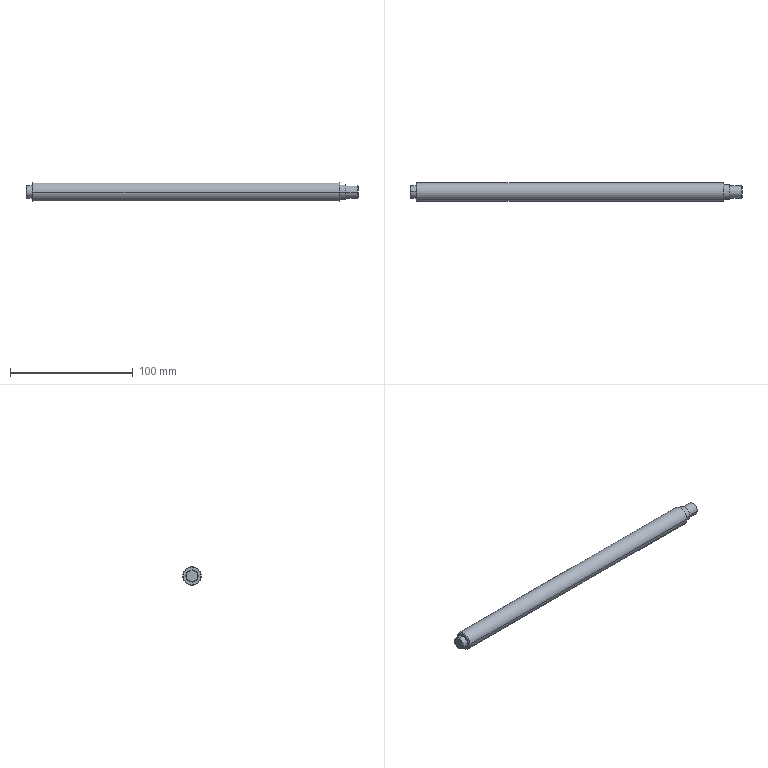Part | STEP file | Guide wheel mechanism revised.sldasm-Part-351 | 1 solid | 19 faces | box 270 x 15 x 15 mm | volume 45909 mm3 | cylinder 8 | cone 6 | plane 5 | commonest cylinder face diameters 10 x4 12 x2 15 x2
STEP:
#1=CARTESIAN_POINT('',(0.,0.,4.5));
#2=VERTEX_POINT('',#1);
#3=CARTESIAN_POINT('',(0.,0.,-4.5));
#4=VERTEX_POINT('',#3);
#5=CARTESIAN_POINT('',(0.,0.,0.));
#6=DIRECTION('',(-1.,0.,0.));
#7=DIRECTION('',(0.,1.,0.));
#8=AXIS2_PLACEMENT_3D('',#5,#6,#7);
#9=CIRCLE('',#8,4.5);
#10=EDGE_CURVE('',#2,#4,#9,.T.);
#11=ORIENTED_EDGE('',*,*,#10,.F.);
#12=CARTESIAN_POINT('',(0.5,0.,5.));
#13=VERTEX_POINT('',#12);
#14=CARTESIAN_POINT('',(0.,0.,4.5));
#15=DIRECTION('',(0.7071,0.,0.7071));
#16=VECTOR('',#15,1000.);
#17=LINE('',#14,#16);
#18=EDGE_CURVE('',#2,#13,#17,.T.);
#19=ORIENTED_EDGE('',*,*,#18,.T.);
#20=CARTESIAN_POINT('',(0.5,0.,-5.));
#21=VERTEX_POINT('',#20);
#22=CARTESIAN_POINT('',(0.5,0.,0.));
#23=DIRECTION('',(1.,0.,0.));
#24=DIRECTION('',(0.,0.,-1.));
#25=AXIS2_PLACEMENT_3D('',#22,#23,#24);
#26=CIRCLE('',#25,5.);
#27=EDGE_CURVE('',#21,#13,#26,.T.);
#28=ORIENTED_EDGE('',*,*,#27,.F.);
#29=CARTESIAN_POINT('',(0.,0.,-4.5));
#30=DIRECTION('',(0.7071,0.,-0.7071));
#31=VECTOR('',#30,1000.);
#32=LINE('',#29,#31);
#33=EDGE_CURVE('',#4,#21,#32,.T.);
#34=ORIENTED_EDGE('',*,*,#33,.F.);
#35=EDGE_LOOP('',(#11,#19,#28,#34));
#36=FACE_OUTER_BOUND('',#35,.T.);
#37=CARTESIAN_POINT('',(0.,0.,0.));
#38=DIRECTION('',(1.,0.,0.));
#39=DIRECTION('',(0.,0.,-1.));
#40=AXIS2_PLACEMENT_3D('',#37,#38,#39);
#41=CONICAL_SURFACE('',#40,4.5,0.7854);
#42=ADVANCED_FACE('',(#36),#41,.T.);
#43=CARTESIAN_POINT('',(5.,-7.,0.));
#44=VERTEX_POINT('',#43);
#45=CARTESIAN_POINT('',(5.,7.,0.));
#46=VERTEX_POINT('',#45);
#47=CARTESIAN_POINT('',(5.,0.,0.));
#48=DIRECTION('',(-1.,0.,0.));
#49=DIRECTION('',(0.,0.,1.));
#50=AXIS2_PLACEMENT_3D('',#47,#48,#49);
#51=CIRCLE('',#50,7.);
#52=EDGE_CURVE('',#44,#46,#51,.T.);
#53=ORIENTED_EDGE('',*,*,#52,.F.);
#54=CARTESIAN_POINT('',(5.5,-7.5,0.));
#55=VERTEX_POINT('',#54);
#56=CARTESIAN_POINT('',(5.,-7.,0.));
#57=DIRECTION('',(0.7071,-0.7071,0.));
#58=VECTOR('',#57,1000.);
#59=LINE('',#56,#58);
#60=EDGE_CURVE('',#44,#55,#59,.T.);
#61=ORIENTED_EDGE('',*,*,#60,.T.);
#62=CARTESIAN_POINT('',(5.5,7.5,0.));
#63=VERTEX_POINT('',#62);
#64=CARTESIAN_POINT('',(5.5,0.,0.));
#65=DIRECTION('',(1.,0.,0.));
#66=DIRECTION('',(0.,-1.,0.));
#67=AXIS2_PLACEMENT_3D('',#64,#65,#66);
#68=CIRCLE('',#67,7.5);
#69=EDGE_CURVE('',#63,#55,#68,.T.);
#70=ORIENTED_EDGE('',*,*,#69,.F.);
#71=CARTESIAN_POINT('',(5.,7.,0.));
#72=DIRECTION('',(0.7071,0.7071,0.));
#73=VECTOR('',#72,1000.);
#74=LINE('',#71,#73);
#75=EDGE_CURVE('',#46,#63,#74,.T.);
#76=ORIENTED_EDGE('',*,*,#75,.F.);
#77=EDGE_LOOP('',(#53,#61,#70,#76));
#78=FACE_OUTER_BOUND('',#77,.T.);
#79=CARTESIAN_POINT('',(5.,0.,0.));
#80=DIRECTION('',(1.,0.,0.));
#81=DIRECTION('',(0.,1.,0.));
#82=AXIS2_PLACEMENT_3D('',#79,#80,#81);
#83=CONICAL_SURFACE('',#82,7.,0.7854);
#84=ADVANCED_FACE('',(#78),#83,.T.);
#85=CARTESIAN_POINT('',(270.,4.5,0.));
#86=VERTEX_POINT('',#85);
#87=CARTESIAN_POINT('',(270.,-4.5,0.));
#88=VERTEX_POINT('',#87);
#89=CARTESIAN_POINT('',(270.,0.,0.));
#90=DIRECTION('',(1.,0.,0.));
#91=DIRECTION('',(0.,-1.,0.));
#92=AXIS2_PLACEMENT_3D('',#89,#90,#91);
#93=CIRCLE('',#92,4.5);
#94=EDGE_CURVE('',#86,#88,#93,.T.);
#95=ORIENTED_EDGE('',*,*,#94,.F.);
#96=CARTESIAN_POINT('',(269.5,5.,0.));
#97=VERTEX_POINT('',#96);
#98=CARTESIAN_POINT('',(269.5,5.,0.));
#99=DIRECTION('',(-0.7071,0.7071,0.));
#100=VECTOR('',#99,1000.);
#101=LINE('',#98,#100);
#102=EDGE_CURVE('',#86,#97,#101,.T.);
#103=ORIENTED_EDGE('',*,*,#102,.T.);
#104=CARTESIAN_POINT('',(269.5,-5.,0.));
#105=VERTEX_POINT('',#104);
#106=CARTESIAN_POINT('',(269.5,0.,0.));
#107=DIRECTION('',(-1.,0.,0.));
#108=DIRECTION('',(0.,-1.,0.));
#109=AXIS2_PLACEMENT_3D('',#106,#107,#108);
#110=CIRCLE('',#109,5.);
#111=EDGE_CURVE('',#105,#97,#110,.T.);
#112=ORIENTED_EDGE('',*,*,#111,.F.);
#113=CARTESIAN_POINT('',(269.5,-5.,0.));
#114=DIRECTION('',(-0.7071,-0.7071,0.));
#115=VECTOR('',#114,1000.);
#116=LINE('',#113,#115);
#117=EDGE_CURVE('',#88,#105,#116,.T.);
#118=ORIENTED_EDGE('',*,*,#117,.F.);
#119=EDGE_LOOP('',(#95,#103,#112,#118));
#120=FACE_OUTER_BOUND('',#119,.T.);
#121=CARTESIAN_POINT('',(269.5,0.,0.));
#122=DIRECTION('',(-1.,0.,0.));
#123=DIRECTION('',(0.,-1.,0.));
#124=AXIS2_PLACEMENT_3D('',#121,#122,#123);
#125=CONICAL_SURFACE('',#124,5.,0.7854);
#126=ADVANCED_FACE('',(#120),#125,.T.);
#127=CARTESIAN_POINT('',(5.,0.,5.));
#128=VERTEX_POINT('',#127);
#129=CARTESIAN_POINT('',(5.,0.,-5.));
#130=VERTEX_POINT('',#129);
#131=CARTESIAN_POINT('',(5.,0.,0.));
#132=DIRECTION('',(-1.,0.,0.));
#133=DIRECTION('',(0.,0.,1.));
#134=AXIS2_PLACEMENT_3D('',#131,#132,#133);
#135=CIRCLE('',#134,5.);
#136=EDGE_CURVE('',#128,#130,#135,.T.);
#137=ORIENTED_EDGE('',*,*,#136,.T.);
#138=CARTESIAN_POINT('',(12.,0.,-5.));
#139=DIRECTION('',(-1.,0.,0.));
#140=VECTOR('',#139,1000.);
#141=LINE('',#138,#140);
#142=EDGE_CURVE('',#130,#21,#141,.T.);
#143=ORIENTED_EDGE('',*,*,#142,.T.);
#144=ORIENTED_EDGE('',*,*,#27,.T.);
#145=CARTESIAN_POINT('',(12.,0.,5.));
#146=DIRECTION('',(-1.,0.,0.));
#147=VECTOR('',#146,1000.);
#148=LINE('',#145,#147);
#149=EDGE_CURVE('',#128,#13,#148,.T.);
#150=ORIENTED_EDGE('',*,*,#149,.F.);
#151=EDGE_LOOP('',(#137,#143,#144,#150));
#152=FACE_OUTER_BOUND('',#151,.T.);
#153=CARTESIAN_POINT('',(12.,0.,0.));
#154=DIRECTION('',(-1.,0.,0.));
#155=DIRECTION('',(0.,0.,1.));
#156=AXIS2_PLACEMENT_3D('',#153,#154,#155);
#157=CYLINDRICAL_SURFACE('',#156,5.);
#158=ADVANCED_FACE('',(#152),#157,.T.);
#159=ORIENTED_EDGE('',*,*,#111,.T.);
#160=CARTESIAN_POINT('',(260.,5.,0.));
#161=VERTEX_POINT('',#160);
#162=CARTESIAN_POINT('',(270.,5.,0.));
#163=DIRECTION('',(-1.,0.,0.));
#164=VECTOR('',#163,1000.);
#165=LINE('',#162,#164);
#166=EDGE_CURVE('',#97,#161,#165,.T.);
#167=ORIENTED_EDGE('',*,*,#166,.T.);
#168=CARTESIAN_POINT('',(260.,-5.,0.));
#169=VERTEX_POINT('',#168);
#170=CARTESIAN_POINT('',(260.,0.,0.));
#171=DIRECTION('',(-1.,0.,0.));
#172=DIRECTION('',(0.,-1.,0.));
#173=AXIS2_PLACEMENT_3D('',#170,#171,#172);
#174=CIRCLE('',#173,5.);
#175=EDGE_CURVE('',#169,#161,#174,.T.);
#176=ORIENTED_EDGE('',*,*,#175,.F.);
#177=CARTESIAN_POINT('',(270.,-5.,0.));
#178=DIRECTION('',(-1.,0.,0.));
#179=VECTOR('',#178,1000.);
#180=LINE('',#177,#179);
#181=EDGE_CURVE('',#105,#169,#180,.T.);
#182=ORIENTED_EDGE('',*,*,#181,.F.);
#183=EDGE_LOOP('',(#159,#167,#176,#182));
#184=FACE_OUTER_BOUND('',#183,.T.);
#185=CARTESIAN_POINT('',(270.,0.,0.));
#186=DIRECTION('',(-1.,0.,0.));
#187=DIRECTION('',(0.,-1.,0.));
#188=AXIS2_PLACEMENT_3D('',#185,#186,#187);
#189=CYLINDRICAL_SURFACE('',#188,5.);
#190=ADVANCED_FACE('',(#184),#189,.T.);
#191=CARTESIAN_POINT('',(260.,-6.,0.));
#192=VERTEX_POINT('',#191);
#193=CARTESIAN_POINT('',(260.,6.,0.));
#194=VERTEX_POINT('',#193);
#195=CARTESIAN_POINT('',(260.,0.,0.));
#196=DIRECTION('',(-1.,0.,0.));
#197=DIRECTION('',(0.,-1.,0.));
#198=AXIS2_PLACEMENT_3D('',#195,#196,#197);
#199=CIRCLE('',#198,6.);
#200=EDGE_CURVE('',#192,#194,#199,.T.);
#201=ORIENTED_EDGE('',*,*,#200,.T.);
#202=CARTESIAN_POINT('',(255.,6.,0.));
#203=VERTEX_POINT('',#202);
#204=CARTESIAN_POINT('',(270.,6.,0.));
#205=DIRECTION('',(-1.,0.,0.));
#206=VECTOR('',#205,1000.);
#207=LINE('',#204,#206);
#208=EDGE_CURVE('',#194,#203,#207,.T.);
#209=ORIENTED_EDGE('',*,*,#208,.T.);
#210=CARTESIAN_POINT('',(255.,-6.,0.));
#211=VERTEX_POINT('',#210);
#212=CARTESIAN_POINT('',(255.,0.,0.));
#213=DIRECTION('',(-1.,0.,0.));
#214=DIRECTION('',(0.,-1.,0.));
#215=AXIS2_PLACEMENT_3D('',#212,#213,#214);
#216=CIRCLE('',#215,6.);
#217=EDGE_CURVE('',#211,#203,#216,.T.);
#218=ORIENTED_EDGE('',*,*,#217,.F.);
#219=CARTESIAN_POINT('',(270.,-6.,0.));
#220=DIRECTION('',(-1.,0.,0.));
#221=VECTOR('',#220,1000.);
#222=LINE('',#219,#221);
#223=EDGE_CURVE('',#192,#211,#222,.T.);
#224=ORIENTED_EDGE('',*,*,#223,.F.);
#225=EDGE_LOOP('',(#201,#209,#218,#224));
#226=FACE_OUTER_BOUND('',#225,.T.);
#227=CARTESIAN_POINT('',(270.,0.,0.));
#228=DIRECTION('',(-1.,0.,0.));
#229=DIRECTION('',(0.,-1.,0.));
#230=AXIS2_PLACEMENT_3D('',#227,#228,#229);
#231=CYLINDRICAL_SURFACE('',#230,6.);
#232=ADVANCED_FACE('',(#226),#231,.T.);
#233=CARTESIAN_POINT('',(255.,-7.5,0.));
#234=VERTEX_POINT('',#233);
#235=CARTESIAN_POINT('',(255.,7.5,0.));
#236=VERTEX_POINT('',#235);
#237=CARTESIAN_POINT('',(255.,0.,0.));
#238=DIRECTION('',(-1.,0.,0.));
#239=DIRECTION('',(0.,-1.,0.));
#240=AXIS2_PLACEMENT_3D('',#237,#238,#239);
#241=CIRCLE('',#240,7.5);
#242=EDGE_CURVE('',#234,#236,#241,.T.);
#243=ORIENTED_EDGE('',*,*,#242,.T.);
#244=CARTESIAN_POINT('',(270.,7.5,0.));
#245=DIRECTION('',(-1.,0.,0.));
#246=VECTOR('',#245,1000.);
#247=LINE('',#244,#246);
#248=EDGE_CURVE('',#236,#63,#247,.T.);
#249=ORIENTED_EDGE('',*,*,#248,.T.);
#250=ORIENTED_EDGE('',*,*,#69,.T.);
#251=CARTESIAN_POINT('',(270.,-7.5,0.));
#252=DIRECTION('',(-1.,0.,0.));
#253=VECTOR('',#252,1000.);
#254=LINE('',#251,#253);
#255=EDGE_CURVE('',#234,#55,#254,.T.);
#256=ORIENTED_EDGE('',*,*,#255,.F.);
#257=EDGE_LOOP('',(#243,#249,#250,#256));
#258=FACE_OUTER_BOUND('',#257,.T.);
#259=CARTESIAN_POINT('',(270.,0.,0.));
#260=DIRECTION('',(-1.,0.,0.));
#261=DIRECTION('',(0.,-1.,0.));
#262=AXIS2_PLACEMENT_3D('',#259,#260,#261);
#263=CYLINDRICAL_SURFACE('',#262,7.5);
#264=ADVANCED_FACE('',(#258),#263,.T.);
#265=ORIENTED_EDGE('',*,*,#248,.F.);
#266=CARTESIAN_POINT('',(255.,0.,0.));
#267=DIRECTION('',(-1.,0.,0.));
#268=DIRECTION('',(0.,-1.,0.));
#269=AXIS2_PLACEMENT_3D('',#266,#267,#268);
#270=CIRCLE('',#269,7.5);
#271=EDGE_CURVE('',#236,#234,#270,.T.);
#272=ORIENTED_EDGE('',*,*,#271,.T.);
#273=ORIENTED_EDGE('',*,*,#255,.T.);
#274=CARTESIAN_POINT('',(5.5,0.,0.));
#275=DIRECTION('',(1.,0.,0.));
#276=DIRECTION('',(0.,-1.,0.));
#277=AXIS2_PLACEMENT_3D('',#274,#275,#276);
#278=CIRCLE('',#277,7.5);
#279=EDGE_CURVE('',#55,#63,#278,.T.);
#280=ORIENTED_EDGE('',*,*,#279,.T.);
#281=EDGE_LOOP('',(#265,#272,#273,#280));
#282=FACE_OUTER_BOUND('',#281,.T.);
#283=CARTESIAN_POINT('',(270.,0.,0.));
#284=DIRECTION('',(-1.,0.,0.));
#285=DIRECTION('',(0.,-1.,0.));
#286=AXIS2_PLACEMENT_3D('',#283,#284,#285);
#287=CYLINDRICAL_SURFACE('',#286,7.5);
#288=ADVANCED_FACE('',(#282),#287,.T.);
#289=ORIENTED_EDGE('',*,*,#242,.F.);
#290=ORIENTED_EDGE('',*,*,#271,.F.);
#291=EDGE_LOOP('',(#289,#290));
#292=FACE_OUTER_BOUND('',#291,.T.);
#293=ORIENTED_EDGE('',*,*,#217,.T.);
#294=CARTESIAN_POINT('',(255.,0.,0.));
#295=DIRECTION('',(-1.,0.,0.));
#296=DIRECTION('',(0.,-1.,0.));
#297=AXIS2_PLACEMENT_3D('',#294,#295,#296);
#298=CIRCLE('',#297,6.);
#299=EDGE_CURVE('',#203,#211,#298,.T.);
#300=ORIENTED_EDGE('',*,*,#299,.T.);
#301=EDGE_LOOP('',(#293,#300));
#302=FACE_BOUND('',#301,.T.);
#303=CARTESIAN_POINT('',(255.,7.5,0.));
#304=DIRECTION('',(-1.,0.,0.));
#305=DIRECTION('',(0.,-1.,0.));
#306=AXIS2_PLACEMENT_3D('',#303,#304,#305);
#307=PLANE('',#306);
#308=ADVANCED_FACE('',(#292,#302),#307,.F.);
#309=ORIENTED_EDGE('',*,*,#208,.F.);
#310=CARTESIAN_POINT('',(260.,0.,0.));
#311=DIRECTION('',(-1.,0.,0.));
#312=DIRECTION('',(0.,-1.,0.));
#313=AXIS2_PLACEMENT_3D('',#310,#311,#312);
#314=CIRCLE('',#313,6.);
#315=EDGE_CURVE('',#194,#192,#314,.T.);
#316=ORIENTED_EDGE('',*,*,#315,.T.);
#317=ORIENTED_EDGE('',*,*,#223,.T.);
#318=ORIENTED_EDGE('',*,*,#299,.F.);
#319=EDGE_LOOP('',(#309,#316,#317,#318));
#320=FACE_OUTER_BOUND('',#319,.T.);
#321=CARTESIAN_POINT('',(270.,0.,0.));
#322=DIRECTION('',(-1.,0.,0.));
#323=DIRECTION('',(0.,-1.,0.));
#324=AXIS2_PLACEMENT_3D('',#321,#322,#323);
#325=CYLINDRICAL_SURFACE('',#324,6.);
#326=ADVANCED_FACE('',(#320),#325,.T.);
#327=ORIENTED_EDGE('',*,*,#200,.F.);
#328=ORIENTED_EDGE('',*,*,#315,.F.);
#329=EDGE_LOOP('',(#327,#328));
#330=FACE_OUTER_BOUND('',#329,.T.);
#331=ORIENTED_EDGE('',*,*,#175,.T.);
#332=CARTESIAN_POINT('',(260.,0.,0.));
#333=DIRECTION('',(-1.,0.,0.));
#334=DIRECTION('',(0.,-1.,0.));
#335=AXIS2_PLACEMENT_3D('',#332,#333,#334);
#336=CIRCLE('',#335,5.);
#337=EDGE_CURVE('',#161,#169,#336,.T.);
#338=ORIENTED_EDGE('',*,*,#337,.T.);
#339=EDGE_LOOP('',(#331,#338));
#340=FACE_BOUND('',#339,.T.);
#341=CARTESIAN_POINT('',(260.,6.,0.));
#342=DIRECTION('',(-1.,0.,0.));
#343=DIRECTION('',(0.,-1.,0.));
#344=AXIS2_PLACEMENT_3D('',#341,#342,#343);
#345=PLANE('',#344);
#346=ADVANCED_FACE('',(#330,#340),#345,.F.);
#347=ORIENTED_EDGE('',*,*,#166,.F.);
#348=CARTESIAN_POINT('',(269.5,0.,0.));
#349=DIRECTION('',(-1.,0.,0.));
#350=DIRECTION('',(0.,-1.,0.));
#351=AXIS2_PLACEMENT_3D('',#348,#349,#350);
#352=CIRCLE('',#351,5.);
#353=EDGE_CURVE('',#97,#105,#352,.T.);
#354=ORIENTED_EDGE('',*,*,#353,.T.);
#355=ORIENTED_EDGE('',*,*,#181,.T.);
#356=ORIENTED_EDGE('',*,*,#337,.F.);
#357=EDGE_LOOP('',(#347,#354,#355,#356));
#358=FACE_OUTER_BOUND('',#357,.T.);
#359=CARTESIAN_POINT('',(270.,0.,0.));
#360=DIRECTION('',(-1.,0.,0.));
#361=DIRECTION('',(0.,-1.,0.));
#362=AXIS2_PLACEMENT_3D('',#359,#360,#361);
#363=CYLINDRICAL_SURFACE('',#362,5.);
#364=ADVANCED_FACE('',(#358),#363,.T.);
#365=CARTESIAN_POINT('',(270.,0.,0.));
#366=DIRECTION('',(1.,0.,0.));
#367=DIRECTION('',(0.,-1.,0.));
#368=AXIS2_PLACEMENT_3D('',#365,#366,#367);
#369=CIRCLE('',#368,4.5);
#370=EDGE_CURVE('',#88,#86,#369,.T.);
#371=ORIENTED_EDGE('',*,*,#370,.T.);
#372=ORIENTED_EDGE('',*,*,#94,.T.);
#373=EDGE_LOOP('',(#371,#372));
#374=FACE_OUTER_BOUND('',#373,.T.);
#375=CARTESIAN_POINT('',(270.,5.,0.));
#376=DIRECTION('',(-1.,0.,0.));
#377=DIRECTION('',(0.,-1.,0.));
#378=AXIS2_PLACEMENT_3D('',#375,#376,#377);
#379=PLANE('',#378);
#380=ADVANCED_FACE('',(#374),#379,.F.);
#381=ORIENTED_EDGE('',*,*,#142,.F.);
#382=CARTESIAN_POINT('',(5.,0.,0.));
#383=DIRECTION('',(-1.,0.,0.));
#384=DIRECTION('',(0.,0.,1.));
#385=AXIS2_PLACEMENT_3D('',#382,#383,#384);
#386=CIRCLE('',#385,5.);
#387=EDGE_CURVE('',#130,#128,#386,.T.);
#388=ORIENTED_EDGE('',*,*,#387,.T.);
#389=ORIENTED_EDGE('',*,*,#149,.T.);
#390=CARTESIAN_POINT('',(0.5,0.,0.));
#391=DIRECTION('',(1.,0.,0.));
#392=DIRECTION('',(0.,0.,-1.));
#393=AXIS2_PLACEMENT_3D('',#390,#391,#392);
#394=CIRCLE('',#393,5.);
#395=EDGE_CURVE('',#13,#21,#394,.T.);
#396=ORIENTED_EDGE('',*,*,#395,.T.);
#397=EDGE_LOOP('',(#381,#388,#389,#396));
#398=FACE_OUTER_BOUND('',#397,.T.);
#399=CARTESIAN_POINT('',(12.,0.,0.));
#400=DIRECTION('',(-1.,0.,0.));
#401=DIRECTION('',(0.,0.,1.));
#402=AXIS2_PLACEMENT_3D('',#399,#400,#401);
#403=CYLINDRICAL_SURFACE('',#402,5.);
#404=ADVANCED_FACE('',(#398),#403,.T.);
#405=CARTESIAN_POINT('',(5.,0.,0.));
#406=DIRECTION('',(-1.,0.,0.));
#407=DIRECTION('',(0.,0.,1.));
#408=AXIS2_PLACEMENT_3D('',#405,#406,#407);
#409=CIRCLE('',#408,7.);
#410=EDGE_CURVE('',#46,#44,#409,.T.);
#411=ORIENTED_EDGE('',*,*,#410,.T.);
#412=ORIENTED_EDGE('',*,*,#52,.T.);
#413=EDGE_LOOP('',(#411,#412));
#414=FACE_OUTER_BOUND('',#413,.T.);
#415=ORIENTED_EDGE('',*,*,#136,.F.);
#416=ORIENTED_EDGE('',*,*,#387,.F.);
#417=EDGE_LOOP('',(#415,#416));
#418=FACE_BOUND('',#417,.T.);
#419=CARTESIAN_POINT('',(5.,5.,0.));
#420=DIRECTION('',(-1.,0.,0.));
#421=DIRECTION('',(0.,0.,1.));
#422=AXIS2_PLACEMENT_3D('',#419,#420,#421);
#423=PLANE('',#422);
#424=ADVANCED_FACE('',(#414,#418),#423,.T.);
#425=CARTESIAN_POINT('',(0.,0.,0.));
#426=DIRECTION('',(-1.,0.,0.));
#427=DIRECTION('',(0.,1.,0.));
#428=AXIS2_PLACEMENT_3D('',#425,#426,#427);
#429=CIRCLE('',#428,4.5);
#430=EDGE_CURVE('',#4,#2,#429,.T.);
#431=ORIENTED_EDGE('',*,*,#430,.T.);
#432=ORIENTED_EDGE('',*,*,#10,.T.);
#433=EDGE_LOOP('',(#431,#432));
#434=FACE_OUTER_BOUND('',#433,.T.);
#435=CARTESIAN_POINT('',(0.,0.,0.));
#436=DIRECTION('',(1.,0.,0.));
#437=DIRECTION('',(0.,1.,0.));
#438=AXIS2_PLACEMENT_3D('',#435,#436,#437);
#439=PLANE('',#438);
#440=ADVANCED_FACE('',(#434),#439,.F.);
#441=ORIENTED_EDGE('',*,*,#102,.F.);
#442=ORIENTED_EDGE('',*,*,#370,.F.);
#443=ORIENTED_EDGE('',*,*,#117,.T.);
#444=ORIENTED_EDGE('',*,*,#353,.F.);
#445=EDGE_LOOP('',(#441,#442,#443,#444));
#446=FACE_OUTER_BOUND('',#445,.T.);
#447=CARTESIAN_POINT('',(269.5,0.,0.));
#448=DIRECTION('',(-1.,0.,0.));
#449=DIRECTION('',(0.,-1.,0.));
#450=AXIS2_PLACEMENT_3D('',#447,#448,#449);
#451=CONICAL_SURFACE('',#450,5.,0.7854);
#452=ADVANCED_FACE('',(#446),#451,.T.);
#453=ORIENTED_EDGE('',*,*,#60,.F.);
#454=ORIENTED_EDGE('',*,*,#410,.F.);
#455=ORIENTED_EDGE('',*,*,#75,.T.);
#456=ORIENTED_EDGE('',*,*,#279,.F.);
#457=EDGE_LOOP('',(#453,#454,#455,#456));
#458=FACE_OUTER_BOUND('',#457,.T.);
#459=CARTESIAN_POINT('',(5.,0.,0.));
#460=DIRECTION('',(1.,0.,0.));
#461=DIRECTION('',(0.,1.,0.));
#462=AXIS2_PLACEMENT_3D('',#459,#460,#461);
#463=CONICAL_SURFACE('',#462,7.,0.7854);
#464=ADVANCED_FACE('',(#458),#463,.T.);
#465=ORIENTED_EDGE('',*,*,#18,.F.);
#466=ORIENTED_EDGE('',*,*,#430,.F.);
#467=ORIENTED_EDGE('',*,*,#33,.T.);
#468=ORIENTED_EDGE('',*,*,#395,.F.);
#469=EDGE_LOOP('',(#465,#466,#467,#468));
#470=FACE_OUTER_BOUND('',#469,.T.);
#471=CARTESIAN_POINT('',(0.,0.,0.));
#472=DIRECTION('',(1.,0.,0.));
#473=DIRECTION('',(0.,0.,-1.));
#474=AXIS2_PLACEMENT_3D('',#471,#472,#473);
#475=CONICAL_SURFACE('',#474,4.5,0.7854);
#476=ADVANCED_FACE('',(#470),#475,.T.);
#477=CLOSED_SHELL('',(#42,#84,#126,#158,#190,#232,#264,#288,#308,#326,#346,#364,#380,#404,#424,#440,#452,#464,#476));
#478=MANIFOLD_SOLID_BREP('',#477);
#479=CARTESIAN_POINT('',(0.,0.,0.));
#480=DIRECTION('',(0.,0.,1.));
#481=DIRECTION('',(1.,0.,0.));
#482=AXIS2_PLACEMENT_3D('',#479,#480,#481);
#483=(LENGTH_UNIT()NAMED_UNIT(*)SI_UNIT(.MILLI.,.METRE.));
#484=UNCERTAINTY_MEASURE_WITH_UNIT(LENGTH_MEASURE(0.00001),#483,'','');
#485=(NAMED_UNIT(*)PLANE_ANGLE_UNIT()SI_UNIT($,.RADIAN.));
#486=(NAMED_UNIT(*)SI_UNIT($,.STERADIAN.)SOLID_ANGLE_UNIT());
#487=(GEOMETRIC_REPRESENTATION_CONTEXT(3)GLOBAL_UNCERTAINTY_ASSIGNED_CONTEXT((#484))GLOBAL_UNIT_ASSIGNED_CONTEXT((#483,#485,#486))REPRESENTATION_CONTEXT('',''));
#488=ADVANCED_BREP_SHAPE_REPRESENTATION('',(#478,#482),#487);